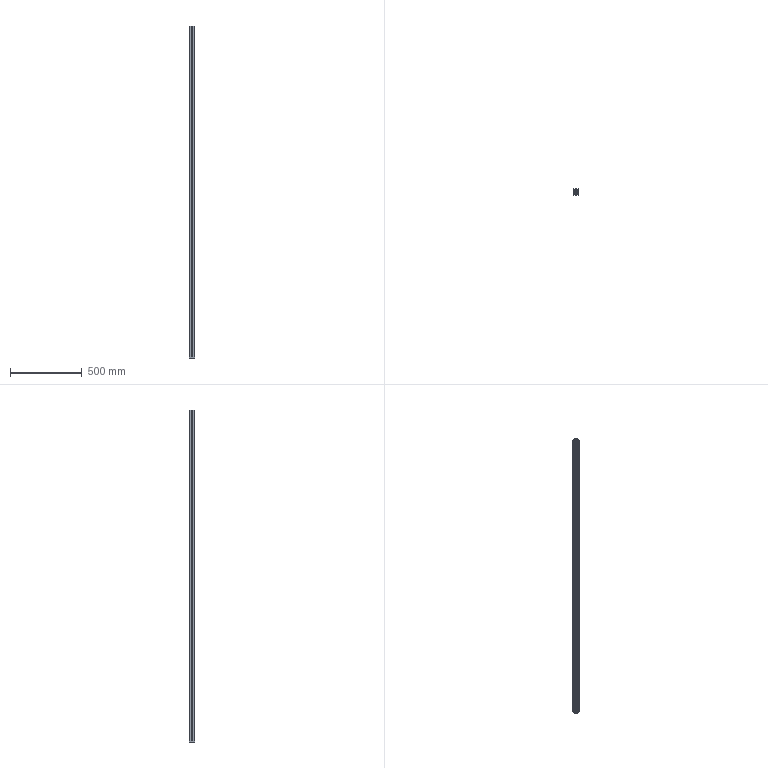Part | SolidWorks | features BaseBody 1 | 1 solid | 273 faces | box 40 x 40 x 2310 mm | volume 1236491 mm3 | plane 186 | cylinder 87 | commonest cylinder face diameters 0.6 x24 9 x16 10 x16 6.8 x15 2 x8 3 x4